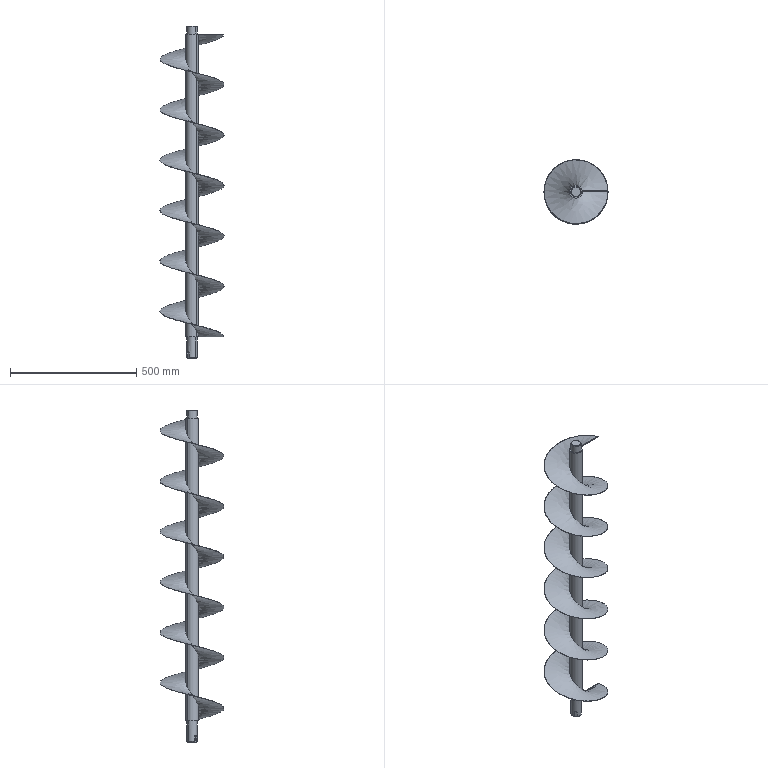Part | SolidWorks | 2 solids | 25 faces | box 253.758 x 253.748 x 1316 mm | volume 2925068 mm3 | plane 9 | cylinder 7 | cone 5 | spline 4 | commonest cylinder face diameters 40 x4 50 x2 12 x1